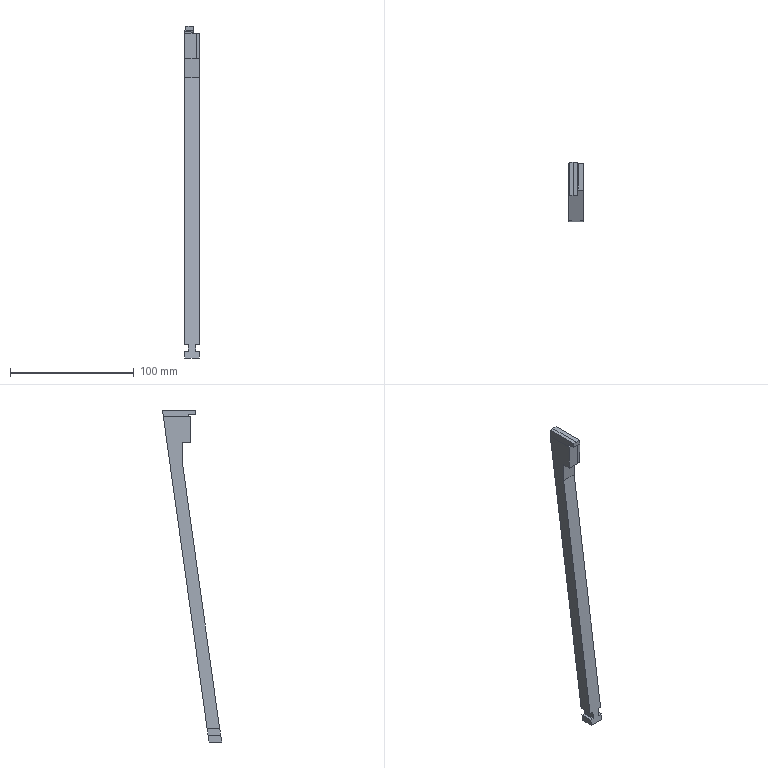Part | Creo | 1 solid | 114 faces | box 12 x 47.744 x 267.86 mm | volume 35083 mm3 | other 63 | plane 45 | cylinder 6 | commonest cylinder face diameters 1 x4 2 x1 12.684 x1